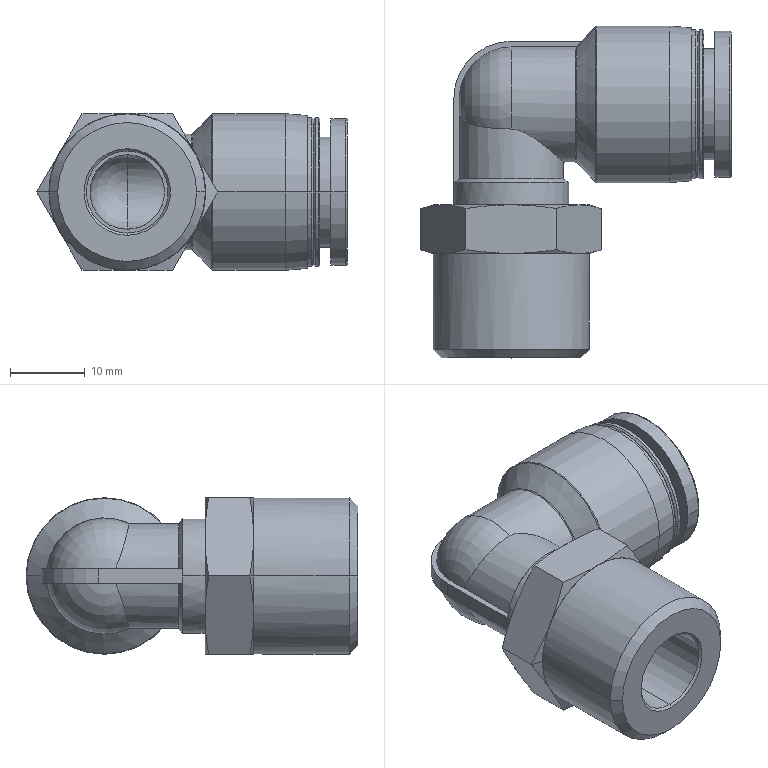Part | SolidWorks | features BaseBody 1 | 1 solid | 92 faces | box 41.624 x 44.5 x 21 mm | volume 11653 mm3 | cone 30 | cylinder 25 | plane 23 | torus 13 | sphere 1 | commonest cylinder face diameters 10 x4 20 x4 15.4 x3 11 x2 12 x2 14.9 x2